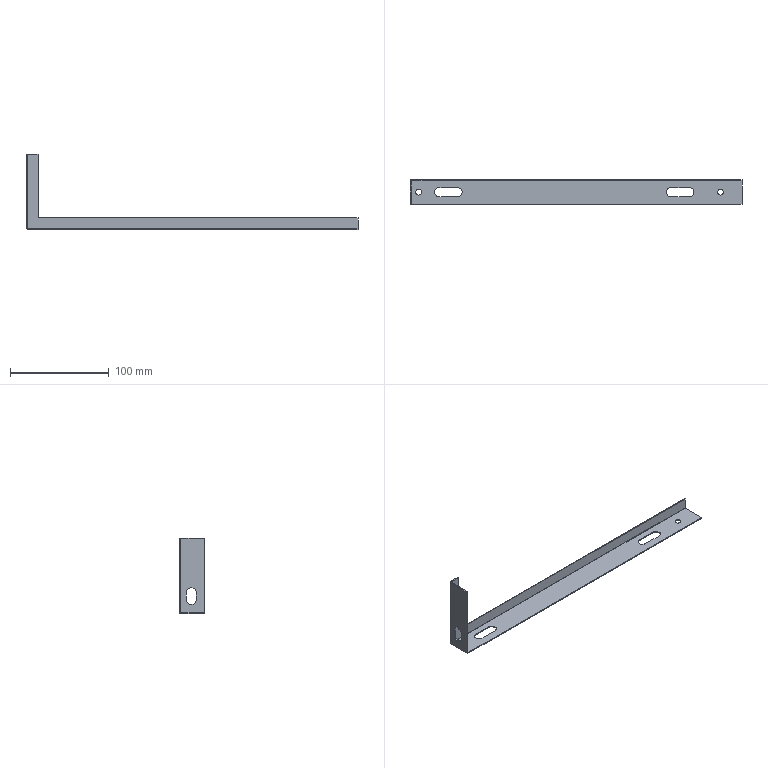Part | SolidWorks | features Cut 2, EdgeFlange 2, FlatPattern 1, ICE 1, LPattern 1, SMBaseFlange 1, SheetMetal 1 | 1 solid | 40 faces | box 336 x 25 x 76.7 mm | volume 13934 mm3 | plane 26 | cylinder 14 | commonest cylinder face diameters 6 x4 9 x4 0.4 x2 2.4 x2 10 x2
STEP:
#1=CARTESIAN_POINT('',(145.7,-15.5,-0.2));
#2=VERTEX_POINT('',#1);
#3=CARTESIAN_POINT('',(145.7,-9.5,-0.2));
#4=VERTEX_POINT('',#3);
#5=CARTESIAN_POINT('',(145.7,-12.5,-0.2));
#6=DIRECTION('',(0.,0.,-1.));
#7=DIRECTION('',(0.,1.,0.));
#8=AXIS2_PLACEMENT_3D('',#5,#6,#7);
#9=CIRCLE('',#8,3.);
#10=EDGE_CURVE('',#2,#4,#9,.T.);
#11=ORIENTED_EDGE('',*,*,#10,.F.);
#12=CARTESIAN_POINT('',(145.7,-15.5,-1.2));
#13=VERTEX_POINT('',#12);
#14=CARTESIAN_POINT('',(145.7,-15.5,8.8));
#15=DIRECTION('',(0.,0.,-1.));
#16=VECTOR('',#15,1000.);
#17=LINE('',#14,#16);
#18=EDGE_CURVE('',#2,#13,#17,.T.);
#19=ORIENTED_EDGE('',*,*,#18,.T.);
#20=CARTESIAN_POINT('',(145.7,-9.5,-1.2));
#21=VERTEX_POINT('',#20);
#22=CARTESIAN_POINT('',(145.7,-12.5,-1.2));
#23=DIRECTION('',(0.,0.,-1.));
#24=DIRECTION('',(0.,1.,0.));
#25=AXIS2_PLACEMENT_3D('',#22,#23,#24);
#26=CIRCLE('',#25,3.);
#27=EDGE_CURVE('',#13,#21,#26,.T.);
#28=ORIENTED_EDGE('',*,*,#27,.T.);
#29=CARTESIAN_POINT('',(145.7,-9.5,8.8));
#30=DIRECTION('',(0.,0.,-1.));
#31=VECTOR('',#30,1000.);
#32=LINE('',#29,#31);
#33=EDGE_CURVE('',#4,#21,#32,.T.);
#34=ORIENTED_EDGE('',*,*,#33,.F.);
#35=EDGE_LOOP('',(#11,#19,#28,#34));
#36=FACE_OUTER_BOUND('',#35,.T.);
#37=CARTESIAN_POINT('',(145.7,-12.5,8.8));
#38=DIRECTION('',(0.,0.,-1.));
#39=DIRECTION('',(0.,1.,0.));
#40=AXIS2_PLACEMENT_3D('',#37,#38,#39);
#41=CYLINDRICAL_SURFACE('',#40,3.);
#42=ADVANCED_FACE('',(#36),#41,.F.);
#43=CARTESIAN_POINT('',(-159.8,-15.5,-0.2));
#44=VERTEX_POINT('',#43);
#45=CARTESIAN_POINT('',(-159.8,-9.5,-0.2));
#46=VERTEX_POINT('',#45);
#47=CARTESIAN_POINT('',(-159.8,-12.5,-0.2));
#48=DIRECTION('',(0.,0.,-1.));
#49=DIRECTION('',(0.,1.,0.));
#50=AXIS2_PLACEMENT_3D('',#47,#48,#49);
#51=CIRCLE('',#50,3.);
#52=EDGE_CURVE('',#44,#46,#51,.T.);
#53=ORIENTED_EDGE('',*,*,#52,.F.);
#54=CARTESIAN_POINT('',(-159.8,-15.5,-1.2));
#55=VERTEX_POINT('',#54);
#56=CARTESIAN_POINT('',(-159.8,-15.5,8.8));
#57=DIRECTION('',(0.,0.,-1.));
#58=VECTOR('',#57,1000.);
#59=LINE('',#56,#58);
#60=EDGE_CURVE('',#44,#55,#59,.T.);
#61=ORIENTED_EDGE('',*,*,#60,.T.);
#62=CARTESIAN_POINT('',(-159.8,-9.5,-1.2));
#63=VERTEX_POINT('',#62);
#64=CARTESIAN_POINT('',(-159.8,-12.5,-1.2));
#65=DIRECTION('',(0.,0.,-1.));
#66=DIRECTION('',(0.,1.,0.));
#67=AXIS2_PLACEMENT_3D('',#64,#65,#66);
#68=CIRCLE('',#67,3.);
#69=EDGE_CURVE('',#55,#63,#68,.T.);
#70=ORIENTED_EDGE('',*,*,#69,.T.);
#71=CARTESIAN_POINT('',(-159.8,-9.5,8.8));
#72=DIRECTION('',(0.,0.,-1.));
#73=VECTOR('',#72,1000.);
#74=LINE('',#71,#73);
#75=EDGE_CURVE('',#46,#63,#74,.T.);
#76=ORIENTED_EDGE('',*,*,#75,.F.);
#77=EDGE_LOOP('',(#53,#61,#70,#76));
#78=FACE_OUTER_BOUND('',#77,.T.);
#79=CARTESIAN_POINT('',(-159.8,-12.5,8.8));
#80=DIRECTION('',(0.,0.,-1.));
#81=DIRECTION('',(0.,1.,0.));
#82=AXIS2_PLACEMENT_3D('',#79,#80,#81);
#83=CYLINDRICAL_SURFACE('',#82,3.);
#84=ADVANCED_FACE('',(#78),#83,.F.);
#85=CARTESIAN_POINT('',(167.4,-1.,11.));
#86=VERTEX_POINT('',#85);
#87=CARTESIAN_POINT('',(-156.4,-1.,11.));
#88=VERTEX_POINT('',#87);
#89=CARTESIAN_POINT('',(-167.4,-1.,11.));
#90=DIRECTION('',(-1.,0.,0.));
#91=VECTOR('',#90,1000.);
#92=LINE('',#89,#91);
#93=EDGE_CURVE('',#86,#88,#92,.T.);
#94=ORIENTED_EDGE('',*,*,#93,.T.);
#95=CARTESIAN_POINT('',(-156.4,-1.,75.5));
#96=VERTEX_POINT('',#95);
#97=CARTESIAN_POINT('',(-156.4,-1.,75.5));
#98=DIRECTION('',(0.,0.,1.));
#99=VECTOR('',#98,1000.);
#100=LINE('',#97,#99);
#101=EDGE_CURVE('',#88,#96,#100,.T.);
#102=ORIENTED_EDGE('',*,*,#101,.T.);
#103=CARTESIAN_POINT('',(-167.4,-1.,75.5));
#104=VERTEX_POINT('',#103);
#105=CARTESIAN_POINT('',(-167.4,-1.,75.5));
#106=DIRECTION('',(1.,0.,0.));
#107=VECTOR('',#106,1000.);
#108=LINE('',#105,#107);
#109=EDGE_CURVE('',#104,#96,#108,.T.);
#110=ORIENTED_EDGE('',*,*,#109,.F.);
#111=CARTESIAN_POINT('',(-167.4,-1.,0.));
#112=VERTEX_POINT('',#111);
#113=CARTESIAN_POINT('',(-167.4,-1.,75.5));
#114=DIRECTION('',(0.,0.,-1.));
#115=VECTOR('',#114,1000.);
#116=LINE('',#113,#115);
#117=EDGE_CURVE('',#104,#112,#116,.T.);
#118=ORIENTED_EDGE('',*,*,#117,.T.);
#119=CARTESIAN_POINT('',(167.4,-1.,0.));
#120=VERTEX_POINT('',#119);
#121=CARTESIAN_POINT('',(-167.4,-1.,0.));
#122=DIRECTION('',(1.,0.,0.));
#123=VECTOR('',#122,1000.);
#124=LINE('',#121,#123);
#125=EDGE_CURVE('',#112,#120,#124,.T.);
#126=ORIENTED_EDGE('',*,*,#125,.T.);
#127=CARTESIAN_POINT('',(167.4,-1.,75.5));
#128=DIRECTION('',(0.,0.,-1.));
#129=VECTOR('',#128,1000.);
#130=LINE('',#127,#129);
#131=EDGE_CURVE('',#86,#120,#130,.T.);
#132=ORIENTED_EDGE('',*,*,#131,.F.);
#133=EDGE_LOOP('',(#94,#102,#110,#118,#126,#132));
#134=FACE_OUTER_BOUND('',#133,.T.);
#135=CARTESIAN_POINT('',(-167.4,-1.,75.5));
#136=DIRECTION('',(0.,1.,0.));
#137=DIRECTION('',(-1.,0.,0.));
#138=AXIS2_PLACEMENT_3D('',#135,#136,#137);
#139=PLANE('',#138);
#140=ADVANCED_FACE('',(#134),#139,.F.);
#141=CARTESIAN_POINT('',(167.4,0.,11.));
#142=VERTEX_POINT('',#141);
#143=CARTESIAN_POINT('',(167.4,-10.,11.));
#144=DIRECTION('',(0.,1.,0.));
#145=VECTOR('',#144,1000.);
#146=LINE('',#143,#145);
#147=EDGE_CURVE('',#86,#142,#146,.T.);
#148=ORIENTED_EDGE('',*,*,#147,.F.);
#149=ORIENTED_EDGE('',*,*,#131,.T.);
#150=CARTESIAN_POINT('',(167.4,0.,0.));
#151=VERTEX_POINT('',#150);
#152=CARTESIAN_POINT('',(167.4,0.,0.));
#153=DIRECTION('',(0.,-1.,0.));
#154=VECTOR('',#153,1000.);
#155=LINE('',#152,#154);
#156=EDGE_CURVE('',#151,#120,#155,.T.);
#157=ORIENTED_EDGE('',*,*,#156,.F.);
#158=CARTESIAN_POINT('',(167.4,0.,75.5));
#159=DIRECTION('',(0.,0.,-1.));
#160=VECTOR('',#159,1000.);
#161=LINE('',#158,#160);
#162=EDGE_CURVE('',#142,#151,#161,.T.);
#163=ORIENTED_EDGE('',*,*,#162,.F.);
#164=EDGE_LOOP('',(#148,#149,#157,#163));
#165=FACE_OUTER_BOUND('',#164,.T.);
#166=CARTESIAN_POINT('',(167.4,0.,75.5));
#167=DIRECTION('',(1.,0.,0.));
#168=DIRECTION('',(0.,0.,-1.));
#169=AXIS2_PLACEMENT_3D('',#166,#167,#168);
#170=PLANE('',#169);
#171=ADVANCED_FACE('',(#165),#170,.T.);
#172=CARTESIAN_POINT('',(-156.4,0.,11.));
#173=VERTEX_POINT('',#172);
#174=CARTESIAN_POINT('',(-156.4,0.,75.5));
#175=VERTEX_POINT('',#174);
#176=CARTESIAN_POINT('',(-156.4,0.,75.5));
#177=DIRECTION('',(0.,0.,1.));
#178=VECTOR('',#177,1000.);
#179=LINE('',#176,#178);
#180=EDGE_CURVE('',#173,#175,#179,.T.);
#181=ORIENTED_EDGE('',*,*,#180,.F.);
#182=CARTESIAN_POINT('',(167.4,0.,11.));
#183=DIRECTION('',(-1.,0.,0.));
#184=VECTOR('',#183,1000.);
#185=LINE('',#182,#184);
#186=EDGE_CURVE('',#142,#173,#185,.T.);
#187=ORIENTED_EDGE('',*,*,#186,.F.);
#188=ORIENTED_EDGE('',*,*,#162,.T.);
#189=CARTESIAN_POINT('',(-167.4,0.,0.));
#190=VERTEX_POINT('',#189);
#191=CARTESIAN_POINT('',(-167.4,0.,0.));
#192=DIRECTION('',(1.,0.,0.));
#193=VECTOR('',#192,1000.);
#194=LINE('',#191,#193);
#195=EDGE_CURVE('',#190,#151,#194,.T.);
#196=ORIENTED_EDGE('',*,*,#195,.F.);
#197=CARTESIAN_POINT('',(-167.4,0.,75.5));
#198=VERTEX_POINT('',#197);
#199=CARTESIAN_POINT('',(-167.4,0.,75.5));
#200=DIRECTION('',(0.,0.,-1.));
#201=VECTOR('',#200,1000.);
#202=LINE('',#199,#201);
#203=EDGE_CURVE('',#198,#190,#202,.T.);
#204=ORIENTED_EDGE('',*,*,#203,.F.);
#205=CARTESIAN_POINT('',(-167.4,0.,75.5));
#206=DIRECTION('',(1.,0.,0.));
#207=VECTOR('',#206,1000.);
#208=LINE('',#205,#207);
#209=EDGE_CURVE('',#198,#175,#208,.T.);
#210=ORIENTED_EDGE('',*,*,#209,.T.);
#211=EDGE_LOOP('',(#181,#187,#188,#196,#204,#210));
#212=FACE_OUTER_BOUND('',#211,.T.);
#213=CARTESIAN_POINT('',(-167.4,0.,75.5));
#214=DIRECTION('',(0.,1.,0.));
#215=DIRECTION('',(-1.,0.,0.));
#216=AXIS2_PLACEMENT_3D('',#213,#214,#215);
#217=PLANE('',#216);
#218=ADVANCED_FACE('',(#212),#217,.T.);
#219=ORIENTED_EDGE('',*,*,#109,.T.);
#220=CARTESIAN_POINT('',(-156.4,0.,75.5));
#221=DIRECTION('',(0.,1.,0.));
#222=VECTOR('',#221,1000.);
#223=LINE('',#220,#222);
#224=EDGE_CURVE('',#96,#175,#223,.T.);
#225=ORIENTED_EDGE('',*,*,#224,.T.);
#226=ORIENTED_EDGE('',*,*,#209,.F.);
#227=CARTESIAN_POINT('',(-167.4,-1.,75.5));
#228=DIRECTION('',(0.,1.,0.));
#229=VECTOR('',#228,1000.);
#230=LINE('',#227,#229);
#231=EDGE_CURVE('',#104,#198,#230,.T.);
#232=ORIENTED_EDGE('',*,*,#231,.F.);
#233=EDGE_LOOP('',(#219,#225,#226,#232));
#234=FACE_OUTER_BOUND('',#233,.T.);
#235=CARTESIAN_POINT('',(0.,0.,75.5));
#236=DIRECTION('',(0.,0.,-1.));
#237=DIRECTION('',(-1.,0.,0.));
#238=AXIS2_PLACEMENT_3D('',#235,#236,#237);
#239=PLANE('',#238);
#240=ADVANCED_FACE('',(#234),#239,.F.);
#241=ORIENTED_EDGE('',*,*,#147,.T.);
#242=ORIENTED_EDGE('',*,*,#186,.T.);
#243=CARTESIAN_POINT('',(-156.4,-10.,11.));
#244=DIRECTION('',(0.,1.,0.));
#245=VECTOR('',#244,1000.);
#246=LINE('',#243,#245);
#247=EDGE_CURVE('',#88,#173,#246,.T.);
#248=ORIENTED_EDGE('',*,*,#247,.F.);
#249=ORIENTED_EDGE('',*,*,#93,.F.);
#250=EDGE_LOOP('',(#241,#242,#248,#249));
#251=FACE_OUTER_BOUND('',#250,.T.);
#252=CARTESIAN_POINT('',(167.4,-10.,11.));
#253=DIRECTION('',(0.,0.,-1.));
#254=DIRECTION('',(-1.,0.,0.));
#255=AXIS2_PLACEMENT_3D('',#252,#253,#254);
#256=PLANE('',#255);
#257=ADVANCED_FACE('',(#251),#256,.F.);
#258=ORIENTED_EDGE('',*,*,#247,.T.);
#259=ORIENTED_EDGE('',*,*,#180,.T.);
#260=ORIENTED_EDGE('',*,*,#224,.F.);
#261=ORIENTED_EDGE('',*,*,#101,.F.);
#262=EDGE_LOOP('',(#258,#259,#260,#261));
#263=FACE_OUTER_BOUND('',#262,.T.);
#264=CARTESIAN_POINT('',(-156.4,-10.,75.5));
#265=DIRECTION('',(-1.,0.,0.));
#266=DIRECTION('',(0.,0.,1.));
#267=AXIS2_PLACEMENT_3D('',#264,#265,#266);
#268=PLANE('',#267);
#269=ADVANCED_FACE('',(#263),#268,.F.);
#270=CARTESIAN_POINT('',(-167.4,-1.2,-0.2));
#271=VERTEX_POINT('',#270);
#272=CARTESIAN_POINT('',(-167.4,-1.2,-1.2));
#273=VERTEX_POINT('',#272);
#274=CARTESIAN_POINT('',(-167.4,-1.2,-1.2));
#275=DIRECTION('',(0.,0.,-1.));
#276=VECTOR('',#275,1000.);
#277=LINE('',#274,#276);
#278=EDGE_CURVE('',#271,#273,#277,.T.);
#279=ORIENTED_EDGE('',*,*,#278,.F.);
#280=CARTESIAN_POINT('',(-167.4,-1.2,0.));
#281=DIRECTION('',(-1.,0.,0.));
#282=DIRECTION('',(0.,1.,0.));
#283=AXIS2_PLACEMENT_3D('',#280,#281,#282);
#284=CIRCLE('',#283,0.2);
#285=EDGE_CURVE('',#112,#271,#284,.T.);
#286=ORIENTED_EDGE('',*,*,#285,.F.);
#287=CARTESIAN_POINT('',(-167.4,-1.,0.));
#288=DIRECTION('',(0.,1.,0.));
#289=VECTOR('',#288,1000.);
#290=LINE('',#287,#289);
#291=EDGE_CURVE('',#112,#190,#290,.T.);
#292=ORIENTED_EDGE('',*,*,#291,.T.);
#293=CARTESIAN_POINT('',(-167.4,-1.2,0.));
#294=DIRECTION('',(-1.,0.,0.));
#295=DIRECTION('',(0.,1.,0.));
#296=AXIS2_PLACEMENT_3D('',#293,#294,#295);
#297=CIRCLE('',#296,1.2);
#298=EDGE_CURVE('',#190,#273,#297,.T.);
#299=ORIENTED_EDGE('',*,*,#298,.T.);
#300=EDGE_LOOP('',(#279,#286,#292,#299));
#301=FACE_OUTER_BOUND('',#300,.T.);
#302=CARTESIAN_POINT('',(-167.4,-1.2,0.));
#303=DIRECTION('',(-1.,0.,0.));
#304=DIRECTION('',(0.,-1.,0.));
#305=AXIS2_PLACEMENT_3D('',#302,#303,#304);
#306=PLANE('',#305);
#307=ADVANCED_FACE('',(#301),#306,.T.);
#308=CARTESIAN_POINT('',(167.4,-1.2,-0.2));
#309=VERTEX_POINT('',#308);
#310=CARTESIAN_POINT('',(167.4,-1.2,0.));
#311=DIRECTION('',(1.,0.,0.));
#312=DIRECTION('',(0.,1.,0.));
#313=AXIS2_PLACEMENT_3D('',#310,#311,#312);
#314=CIRCLE('',#313,0.2);
#315=EDGE_CURVE('',#309,#120,#314,.T.);
#316=ORIENTED_EDGE('',*,*,#315,.F.);
#317=CARTESIAN_POINT('',(167.4,-1.2,-1.2));
#318=VERTEX_POINT('',#317);
#319=CARTESIAN_POINT('',(167.4,-1.2,-0.2));
#320=DIRECTION('',(0.,0.,-1.));
#321=VECTOR('',#320,1000.);
#322=LINE('',#319,#321);
#323=EDGE_CURVE('',#309,#318,#322,.T.);
#324=ORIENTED_EDGE('',*,*,#323,.T.);
#325=CARTESIAN_POINT('',(167.4,-1.2,0.));
#326=DIRECTION('',(1.,0.,0.));
#327=DIRECTION('',(0.,1.,0.));
#328=AXIS2_PLACEMENT_3D('',#325,#326,#327);
#329=CIRCLE('',#328,1.2);
#330=EDGE_CURVE('',#318,#151,#329,.T.);
#331=ORIENTED_EDGE('',*,*,#330,.T.);
#332=ORIENTED_EDGE('',*,*,#156,.T.);
#333=EDGE_LOOP('',(#316,#324,#331,#332));
#334=FACE_OUTER_BOUND('',#333,.T.);
#335=CARTESIAN_POINT('',(167.4,-1.2,0.));
#336=DIRECTION('',(-1.,0.,0.));
#337=DIRECTION('',(0.,-1.,0.));
#338=AXIS2_PLACEMENT_3D('',#335,#336,#337);
#339=PLANE('',#338);
#340=ADVANCED_FACE('',(#334),#339,.F.);
#341=ORIENTED_EDGE('',*,*,#195,.T.);
#342=ORIENTED_EDGE('',*,*,#330,.F.);
#343=CARTESIAN_POINT('',(0.,-1.2,-1.2));
#344=DIRECTION('',(1.,0.,0.));
#345=VECTOR('',#344,1000.);
#346=LINE('',#343,#345);
#347=EDGE_CURVE('',#273,#318,#346,.T.);
#348=ORIENTED_EDGE('',*,*,#347,.F.);
#349=ORIENTED_EDGE('',*,*,#298,.F.);
#350=EDGE_LOOP('',(#341,#342,#348,#349));
#351=FACE_OUTER_BOUND('',#350,.T.);
#352=CARTESIAN_POINT('',(167.4,-1.2,0.));
#353=DIRECTION('',(1.,0.,0.));
#354=DIRECTION('',(0.,0.,-1.));
#355=AXIS2_PLACEMENT_3D('',#352,#353,#354);
#356=CYLINDRICAL_SURFACE('',#355,1.2);
#357=ADVANCED_FACE('',(#351),#356,.T.);
#358=ORIENTED_EDGE('',*,*,#125,.F.);
#359=ORIENTED_EDGE('',*,*,#285,.T.);
#360=CARTESIAN_POINT('',(-167.4,-1.2,-0.2));
#361=DIRECTION('',(1.,0.,0.));
#362=VECTOR('',#361,1000.);
#363=LINE('',#360,#362);
#364=EDGE_CURVE('',#271,#309,#363,.T.);
#365=ORIENTED_EDGE('',*,*,#364,.T.);
#366=ORIENTED_EDGE('',*,*,#315,.T.);
#367=EDGE_LOOP('',(#358,#359,#365,#366));
#368=FACE_OUTER_BOUND('',#367,.T.);
#369=CARTESIAN_POINT('',(167.4,-1.2,0.));
#370=DIRECTION('',(1.,0.,0.));
#371=DIRECTION('',(0.,0.,-1.));
#372=AXIS2_PLACEMENT_3D('',#369,#370,#371);
#373=CYLINDRICAL_SURFACE('',#372,0.2);
#374=ADVANCED_FACE('',(#368),#373,.F.);
#375=CARTESIAN_POINT('',(167.4,-25.,-1.2));
#376=VERTEX_POINT('',#375);
#377=CARTESIAN_POINT('',(167.4,-1.,-1.2));
#378=DIRECTION('',(0.,1.,0.));
#379=VECTOR('',#378,1000.);
#380=LINE('',#377,#379);
#381=EDGE_CURVE('',#376,#318,#380,.T.);
#382=ORIENTED_EDGE('',*,*,#381,.T.);
#383=ORIENTED_EDGE('',*,*,#323,.F.);
#384=CARTESIAN_POINT('',(167.4,-25.,-0.2));
#385=VERTEX_POINT('',#384);
#386=CARTESIAN_POINT('',(167.4,0.,-0.2));
#387=DIRECTION('',(0.,1.,0.));
#388=VECTOR('',#387,1000.);
#389=LINE('',#386,#388);
#390=EDGE_CURVE('',#385,#309,#389,.T.);
#391=ORIENTED_EDGE('',*,*,#390,.F.);
#392=CARTESIAN_POINT('',(167.4,-25.,-1.2));
#393=DIRECTION('',(0.,0.,1.));
#394=VECTOR('',#393,1000.);
#395=LINE('',#392,#394);
#396=EDGE_CURVE('',#376,#385,#395,.T.);
#397=ORIENTED_EDGE('',*,*,#396,.F.);
#398=EDGE_LOOP('',(#382,#383,#391,#397));
#399=FACE_OUTER_BOUND('',#398,.T.);
#400=CARTESIAN_POINT('',(167.4,-1.,-1.2));
#401=DIRECTION('',(1.,0.,0.));
#402=DIRECTION('',(0.,0.,-1.));
#403=AXIS2_PLACEMENT_3D('',#400,#401,#402);
#404=PLANE('',#403);
#405=ADVANCED_FACE('',(#399),#404,.T.);
#406=CARTESIAN_POINT('',(-167.4,-25.,-0.2));
#407=VERTEX_POINT('',#406);
#408=CARTESIAN_POINT('',(-167.4,0.,-0.2));
#409=DIRECTION('',(0.,-1.,0.));
#410=VECTOR('',#409,1000.);
#411=LINE('',#408,#410);
#412=EDGE_CURVE('',#271,#407,#411,.T.);
#413=ORIENTED_EDGE('',*,*,#412,.F.);
#414=ORIENTED_EDGE('',*,*,#278,.T.);
#415=CARTESIAN_POINT('',(-167.4,-25.,-1.2));
#416=VERTEX_POINT('',#415);
#417=CARTESIAN_POINT('',(-167.4,-25.,-1.2));
#418=DIRECTION('',(0.,-1.,0.));
#419=VECTOR('',#418,1000.);
#420=LINE('',#417,#419);
#421=EDGE_CURVE('',#273,#416,#420,.T.);
#422=ORIENTED_EDGE('',*,*,#421,.T.);
#423=CARTESIAN_POINT('',(-167.4,-25.,-1.2));
#424=DIRECTION('',(0.,0.,1.));
#425=VECTOR('',#424,1000.);
#426=LINE('',#423,#425);
#427=EDGE_CURVE('',#416,#407,#426,.T.);
#428=ORIENTED_EDGE('',*,*,#427,.T.);
#429=EDGE_LOOP('',(#413,#414,#422,#428));
#430=FACE_OUTER_BOUND('',#429,.T.);
#431=CARTESIAN_POINT('',(-167.4,-25.,-1.2));
#432=DIRECTION('',(-1.,0.,0.));
#433=DIRECTION('',(0.,0.,1.));
#434=AXIS2_PLACEMENT_3D('',#431,#432,#433);
#435=PLANE('',#434);
#436=ADVANCED_FACE('',(#430),#435,.T.);
#437=CARTESIAN_POINT('',(145.7,-12.5,-1.2));
#438=DIRECTION('',(0.,0.,-1.));
#439=DIRECTION('',(0.,1.,0.));
#440=AXIS2_PLACEMENT_3D('',#437,#438,#439);
#441=CIRCLE('',#440,3.);
#442=EDGE_CURVE('',#21,#13,#441,.T.);
#443=ORIENTED_EDGE('',*,*,#442,.F.);
#444=ORIENTED_EDGE('',*,*,#27,.F.);
#445=EDGE_LOOP('',(#443,#444));
#446=FACE_BOUND('',#445,.T.);
#447=CARTESIAN_POINT('',(-159.8,-12.5,-1.2));
#448=DIRECTION('',(0.,0.,-1.));
#449=DIRECTION('',(0.,1.,0.));
#450=AXIS2_PLACEMENT_3D('',#447,#448,#449);
#451=CIRCLE('',#450,3.);
#452=EDGE_CURVE('',#63,#55,#451,.T.);
#453=ORIENTED_EDGE('',*,*,#452,.F.);
#454=ORIENTED_EDGE('',*,*,#69,.F.);
#455=EDGE_LOOP('',(#453,#454));
#456=FACE_BOUND('',#455,.T.);
#457=CARTESIAN_POINT('',(95.2,-17.,-1.2));
#458=VERTEX_POINT('',#457);
#459=CARTESIAN_POINT('',(95.2,-8.,-1.2));
#460=VERTEX_POINT('',#459);
#461=CARTESIAN_POINT('',(95.2,-12.5,-1.2));
#462=DIRECTION('',(0.,0.,-1.));
#463=DIRECTION('',(0.,1.,0.));
#464=AXIS2_PLACEMENT_3D('',#461,#462,#463);
#465=CIRCLE('',#464,4.5);
#466=EDGE_CURVE('',#458,#460,#465,.T.);
#467=ORIENTED_EDGE('',*,*,#466,.F.);
#468=CARTESIAN_POINT('',(114.2,-17.,-1.2));
#469=VERTEX_POINT('',#468);
#470=CARTESIAN_POINT('',(95.2,-17.,-1.2));
#471=DIRECTION('',(-1.,0.,0.));
#472=VECTOR('',#471,1000.);
#473=LINE('',#470,#472);
#474=EDGE_CURVE('',#469,#458,#473,.T.);
#475=ORIENTED_EDGE('',*,*,#474,.F.);
#476=CARTESIAN_POINT('',(114.2,-8.,-1.2));
#477=VERTEX_POINT('',#476);
#478=CARTESIAN_POINT('',(114.2,-12.5,-1.2));
#479=DIRECTION('',(0.,0.,-1.));
#480=DIRECTION('',(0.,1.,0.));
#481=AXIS2_PLACEMENT_3D('',#478,#479,#480);
#482=CIRCLE('',#481,4.5);
#483=EDGE_CURVE('',#477,#469,#482,.T.);
#484=ORIENTED_EDGE('',*,*,#483,.F.);
#485=CARTESIAN_POINT('',(95.2,-8.,-1.2));
#486=DIRECTION('',(1.,0.,0.));
#487=VECTOR('',#486,1000.);
#488=LINE('',#485,#487);
#489=EDGE_CURVE('',#460,#477,#488,.T.);
#490=ORIENTED_EDGE('',*,*,#489,.F.);
#491=EDGE_LOOP('',(#467,#475,#484,#490));
#492=FACE_BOUND('',#491,.T.);
#493=CARTESIAN_POINT('',(-139.3,-17.,-1.2));
#494=VERTEX_POINT('',#493);
#495=CARTESIAN_POINT('',(-139.3,-8.,-1.2));
#496=VERTEX_POINT('',#495);
#497=CARTESIAN_POINT('',(-139.3,-12.5,-1.2));
#498=DIRECTION('',(0.,0.,-1.));
#499=DIRECTION('',(0.,1.,0.));
#500=AXIS2_PLACEMENT_3D('',#497,#498,#499);
#501=CIRCLE('',#500,4.5);
#502=EDGE_CURVE('',#494,#496,#501,.T.);
#503=ORIENTED_EDGE('',*,*,#502,.F.);
#504=CARTESIAN_POINT('',(-120.3,-17.,-1.2));
#505=VERTEX_POINT('',#504);
#506=CARTESIAN_POINT('',(-139.3,-17.,-1.2));
#507=DIRECTION('',(-1.,0.,0.));
#508=VECTOR('',#507,1000.);
#509=LINE('',#506,#508);
#510=EDGE_CURVE('',#505,#494,#509,.T.);
#511=ORIENTED_EDGE('',*,*,#510,.F.);
#512=CARTESIAN_POINT('',(-120.3,-8.,-1.2));
#513=VERTEX_POINT('',#512);
#514=CARTESIAN_POINT('',(-120.3,-12.5,-1.2));
#515=DIRECTION('',(0.,0.,-1.));
#516=DIRECTION('',(0.,1.,0.));
#517=AXIS2_PLACEMENT_3D('',#514,#515,#516);
#518=CIRCLE('',#517,4.5);
#519=EDGE_CURVE('',#513,#505,#518,.T.);
#520=ORIENTED_EDGE('',*,*,#519,.F.);
#521=CARTESIAN_POINT('',(-139.3,-8.,-1.2));
#522=DIRECTION('',(1.,0.,0.));
#523=VECTOR('',#522,1000.);
#524=LINE('',#521,#523);
#525=EDGE_CURVE('',#496,#513,#524,.T.);
#526=ORIENTED_EDGE('',*,*,#525,.F.);
#527=EDGE_LOOP('',(#503,#511,#520,#526));
#528=FACE_BOUND('',#527,.T.);
#529=ORIENTED_EDGE('',*,*,#421,.F.);
#530=ORIENTED_EDGE('',*,*,#347,.T.);
#531=ORIENTED_EDGE('',*,*,#381,.F.);
#532=CARTESIAN_POINT('',(167.4,-25.,-1.2));
#533=DIRECTION('',(1.,0.,0.));
#534=VECTOR('',#533,1000.);
#535=LINE('',#532,#534);
#536=EDGE_CURVE('',#416,#376,#535,.T.);
#537=ORIENTED_EDGE('',*,*,#536,.F.);
#538=EDGE_LOOP('',(#529,#530,#531,#537));
#539=FACE_OUTER_BOUND('',#538,.T.);
#540=CARTESIAN_POINT('',(0.,0.,-1.2));
#541=DIRECTION('',(0.,0.,-1.));
#542=DIRECTION('',(0.,1.,0.));
#543=AXIS2_PLACEMENT_3D('',#540,#541,#542);
#544=PLANE('',#543);
#545=ADVANCED_FACE('',(#446,#456,#492,#528,#539),#544,.T.);
#546=CARTESIAN_POINT('',(145.7,-12.5,-0.2));
#547=DIRECTION('',(0.,0.,-1.));
#548=DIRECTION('',(0.,1.,0.));
#549=AXIS2_PLACEMENT_3D('',#546,#547,#548);
#550=CIRCLE('',#549,3.);
#551=EDGE_CURVE('',#4,#2,#550,.T.);
#552=ORIENTED_EDGE('',*,*,#551,.T.);
#553=ORIENTED_EDGE('',*,*,#10,.T.);
#554=EDGE_LOOP('',(#552,#553));
#555=FACE_BOUND('',#554,.T.);
#556=CARTESIAN_POINT('',(-159.8,-12.5,-0.2));
#557=DIRECTION('',(0.,0.,-1.));
#558=DIRECTION('',(0.,1.,0.));
#559=AXIS2_PLACEMENT_3D('',#556,#557,#558);
#560=CIRCLE('',#559,3.);
#561=EDGE_CURVE('',#46,#44,#560,.T.);
#562=ORIENTED_EDGE('',*,*,#561,.T.);
#563=ORIENTED_EDGE('',*,*,#52,.T.);
#564=EDGE_LOOP('',(#562,#563));
#565=FACE_BOUND('',#564,.T.);
#566=CARTESIAN_POINT('',(114.2,-17.,-0.2));
#567=VERTEX_POINT('',#566);
#568=CARTESIAN_POINT('',(95.2,-17.,-0.2));
#569=VERTEX_POINT('',#568);
#570=CARTESIAN_POINT('',(0.,-17.,-0.2));
#571=DIRECTION('',(-1.,0.,0.));
#572=VECTOR('',#571,1000.);
#573=LINE('',#570,#572);
#574=EDGE_CURVE('',#567,#569,#573,.T.);
#575=ORIENTED_EDGE('',*,*,#574,.T.);
#576=CARTESIAN_POINT('',(95.2,-8.,-0.2));
#577=VERTEX_POINT('',#576);
#578=CARTESIAN_POINT('',(95.2,-12.5,-0.2));
#579=DIRECTION('',(0.,0.,-1.));
#580=DIRECTION('',(0.,1.,0.));
#581=AXIS2_PLACEMENT_3D('',#578,#579,#580);
#582=CIRCLE('',#581,4.5);
#583=EDGE_CURVE('',#569,#577,#582,.T.);
#584=ORIENTED_EDGE('',*,*,#583,.T.);
#585=CARTESIAN_POINT('',(114.2,-8.,-0.2));
#586=VERTEX_POINT('',#585);
#587=CARTESIAN_POINT('',(0.,-8.,-0.2));
#588=DIRECTION('',(1.,0.,0.));
#589=VECTOR('',#588,1000.);
#590=LINE('',#587,#589);
#591=EDGE_CURVE('',#577,#586,#590,.T.);
#592=ORIENTED_EDGE('',*,*,#591,.T.);
#593=CARTESIAN_POINT('',(114.2,-12.5,-0.2));
#594=DIRECTION('',(0.,0.,-1.));
#595=DIRECTION('',(0.,1.,0.));
#596=AXIS2_PLACEMENT_3D('',#593,#594,#595);
#597=CIRCLE('',#596,4.5);
#598=EDGE_CURVE('',#586,#567,#597,.T.);
#599=ORIENTED_EDGE('',*,*,#598,.T.);
#600=EDGE_LOOP('',(#575,#584,#592,#599));
#601=FACE_BOUND('',#600,.T.);
#602=CARTESIAN_POINT('',(-120.3,-17.,-0.2));
#603=VERTEX_POINT('',#602);
#604=CARTESIAN_POINT('',(-139.3,-17.,-0.2));
#605=VERTEX_POINT('',#604);
#606=CARTESIAN_POINT('',(0.,-17.,-0.2));
#607=DIRECTION('',(-1.,0.,0.));
#608=VECTOR('',#607,1000.);
#609=LINE('',#606,#608);
#610=EDGE_CURVE('',#603,#605,#609,.T.);
#611=ORIENTED_EDGE('',*,*,#610,.T.);
#612=CARTESIAN_POINT('',(-139.3,-8.,-0.2));
#613=VERTEX_POINT('',#612);
#614=CARTESIAN_POINT('',(-139.3,-12.5,-0.2));
#615=DIRECTION('',(0.,0.,-1.));
#616=DIRECTION('',(0.,1.,0.));
#617=AXIS2_PLACEMENT_3D('',#614,#615,#616);
#618=CIRCLE('',#617,4.5);
#619=EDGE_CURVE('',#605,#613,#618,.T.);
#620=ORIENTED_EDGE('',*,*,#619,.T.);
#621=CARTESIAN_POINT('',(-120.3,-8.,-0.2));
#622=VERTEX_POINT('',#621);
#623=CARTESIAN_POINT('',(0.,-8.,-0.2));
#624=DIRECTION('',(1.,0.,0.));
#625=VECTOR('',#624,1000.);
#626=LINE('',#623,#625);
#627=EDGE_CURVE('',#613,#622,#626,.T.);
#628=ORIENTED_EDGE('',*,*,#627,.T.);
#629=CARTESIAN_POINT('',(-120.3,-12.5,-0.2));
#630=DIRECTION('',(0.,0.,-1.));
#631=DIRECTION('',(0.,1.,0.));
#632=AXIS2_PLACEMENT_3D('',#629,#630,#631);
#633=CIRCLE('',#632,4.5);
#634=EDGE_CURVE('',#622,#603,#633,.T.);
#635=ORIENTED_EDGE('',*,*,#634,.T.);
#636=EDGE_LOOP('',(#611,#620,#628,#635));
#637=FACE_BOUND('',#636,.T.);
#638=ORIENTED_EDGE('',*,*,#364,.F.);
#639=ORIENTED_EDGE('',*,*,#412,.T.);
#640=CARTESIAN_POINT('',(0.,-25.,-0.2));
#641=DIRECTION('',(1.,0.,0.));
#642=VECTOR('',#641,1000.);
#643=LINE('',#640,#642);
#644=EDGE_CURVE('',#407,#385,#643,.T.);
#645=ORIENTED_EDGE('',*,*,#644,.T.);
#646=ORIENTED_EDGE('',*,*,#390,.T.);
#647=EDGE_LOOP('',(#638,#639,#645,#646));
#648=FACE_OUTER_BOUND('',#647,.T.);
#649=CARTESIAN_POINT('',(0.,0.,-0.2));
#650=DIRECTION('',(0.,0.,-1.));
#651=DIRECTION('',(0.,1.,0.));
#652=AXIS2_PLACEMENT_3D('',#649,#650,#651);
#653=PLANE('',#652);
#654=ADVANCED_FACE('',(#555,#565,#601,#637,#648),#653,.F.);
#655=ORIENTED_EDGE('',*,*,#644,.F.);
#656=ORIENTED_EDGE('',*,*,#427,.F.);
#657=ORIENTED_EDGE('',*,*,#536,.T.);
#658=ORIENTED_EDGE('',*,*,#396,.T.);
#659=EDGE_LOOP('',(#655,#656,#657,#658));
#660=FACE_OUTER_BOUND('',#659,.T.);
#661=CARTESIAN_POINT('',(167.4,-25.,-1.2));
#662=DIRECTION('',(0.,-1.,0.));
#663=DIRECTION('',(0.,0.,-1.));
#664=AXIS2_PLACEMENT_3D('',#661,#662,#663);
#665=PLANE('',#664);
#666=ADVANCED_FACE('',(#660),#665,.T.);
#667=CARTESIAN_POINT('',(-167.6,-1.2,75.5));
#668=VERTEX_POINT('',#667);
#669=CARTESIAN_POINT('',(-168.6,-1.2,75.5));
#670=VERTEX_POINT('',#669);
#671=CARTESIAN_POINT('',(-168.6,-1.2,75.5));
#672=DIRECTION('',(-1.,0.,0.));
#673=VECTOR('',#672,1000.);
#674=LINE('',#671,#673);
#675=EDGE_CURVE('',#668,#670,#674,.T.);
#676=ORIENTED_EDGE('',*,*,#675,.F.);
#677=CARTESIAN_POINT('',(-167.4,-1.2,75.5));
#678=DIRECTION('',(0.,0.,1.));
#679=DIRECTION('',(-1.,0.,0.));
#680=AXIS2_PLACEMENT_3D('',#677,#678,#679);
#681=CIRCLE('',#680,0.2);
#682=EDGE_CURVE('',#104,#668,#681,.T.);
#683=ORIENTED_EDGE('',*,*,#682,.F.);
#684=ORIENTED_EDGE('',*,*,#231,.T.);
#685=CARTESIAN_POINT('',(-167.4,-1.2,75.5));
#686=DIRECTION('',(0.,0.,1.));
#687=DIRECTION('',(-1.,0.,0.));
#688=AXIS2_PLACEMENT_3D('',#685,#686,#687);
#689=CIRCLE('',#688,1.2);
#690=EDGE_CURVE('',#198,#670,#689,.T.);
#691=ORIENTED_EDGE('',*,*,#690,.T.);
#692=EDGE_LOOP('',(#676,#683,#684,#691));
#693=FACE_OUTER_BOUND('',#692,.T.);
#694=CARTESIAN_POINT('',(-167.4,-1.2,75.5));
#695=DIRECTION('',(0.,0.,1.));
#696=DIRECTION('',(1.,0.,0.));
#697=AXIS2_PLACEMENT_3D('',#694,#695,#696);
#698=PLANE('',#697);
#699=ADVANCED_FACE('',(#693),#698,.T.);
#700=CARTESIAN_POINT('',(-167.6,-1.2,0.));
#701=VERTEX_POINT('',#700);
#702=CARTESIAN_POINT('',(-167.4,-1.2,0.));
#703=DIRECTION('',(0.,0.,-1.));
#704=DIRECTION('',(-1.,0.,0.));
#705=AXIS2_PLACEMENT_3D('',#702,#703,#704);
#706=CIRCLE('',#705,0.2);
#707=EDGE_CURVE('',#701,#112,#706,.T.);
#708=ORIENTED_EDGE('',*,*,#707,.F.);
#709=CARTESIAN_POINT('',(-168.6,-1.2,0.));
#710=VERTEX_POINT('',#709);
#711=CARTESIAN_POINT('',(-167.6,-1.2,0.));
#712=DIRECTION('',(-1.,0.,0.));
#713=VECTOR('',#712,1000.);
#714=LINE('',#711,#713);
#715=EDGE_CURVE('',#701,#710,#714,.T.);
#716=ORIENTED_EDGE('',*,*,#715,.T.);
#717=CARTESIAN_POINT('',(-167.4,-1.2,0.));
#718=DIRECTION('',(0.,0.,-1.));
#719=DIRECTION('',(-1.,0.,0.));
#720=AXIS2_PLACEMENT_3D('',#717,#718,#719);
#721=CIRCLE('',#720,1.2);
#722=EDGE_CURVE('',#710,#190,#721,.T.);
#723=ORIENTED_EDGE('',*,*,#722,.T.);
#724=ORIENTED_EDGE('',*,*,#291,.F.);
#725=EDGE_LOOP('',(#708,#716,#723,#724));
#726=FACE_OUTER_BOUND('',#725,.T.);
#727=CARTESIAN_POINT('',(-167.4,-1.2,0.));
#728=DIRECTION('',(0.,0.,1.));
#729=DIRECTION('',(1.,0.,0.));
#730=AXIS2_PLACEMENT_3D('',#727,#728,#729);
#731=PLANE('',#730);
#732=ADVANCED_FACE('',(#726),#731,.F.);
#733=ORIENTED_EDGE('',*,*,#203,.T.);
#734=ORIENTED_EDGE('',*,*,#722,.F.);
#735=CARTESIAN_POINT('',(-168.6,-1.2,0.));
#736=DIRECTION('',(0.,0.,-1.));
#737=VECTOR('',#736,1000.);
#738=LINE('',#735,#737);
#739=EDGE_CURVE('',#670,#710,#738,.T.);
#740=ORIENTED_EDGE('',*,*,#739,.F.);
#741=ORIENTED_EDGE('',*,*,#690,.F.);
#742=EDGE_LOOP('',(#733,#734,#740,#741));
#743=FACE_OUTER_BOUND('',#742,.T.);
#744=CARTESIAN_POINT('',(-167.4,-1.2,0.));
#745=DIRECTION('',(0.,0.,-1.));
#746=DIRECTION('',(-1.,0.,0.));
#747=AXIS2_PLACEMENT_3D('',#744,#745,#746);
#748=CYLINDRICAL_SURFACE('',#747,1.2);
#749=ADVANCED_FACE('',(#743),#748,.T.);
#750=ORIENTED_EDGE('',*,*,#117,.F.);
#751=ORIENTED_EDGE('',*,*,#682,.T.);
#752=CARTESIAN_POINT('',(-167.6,-1.2,75.5));
#753=DIRECTION('',(0.,0.,-1.));
#754=VECTOR('',#753,1000.);
#755=LINE('',#752,#754);
#756=EDGE_CURVE('',#668,#701,#755,.T.);
#757=ORIENTED_EDGE('',*,*,#756,.T.);
#758=ORIENTED_EDGE('',*,*,#707,.T.);
#759=EDGE_LOOP('',(#750,#751,#757,#758));
#760=FACE_OUTER_BOUND('',#759,.T.);
#761=CARTESIAN_POINT('',(-167.4,-1.2,0.));
#762=DIRECTION('',(0.,0.,-1.));
#763=DIRECTION('',(-1.,0.,0.));
#764=AXIS2_PLACEMENT_3D('',#761,#762,#763);
#765=CYLINDRICAL_SURFACE('',#764,0.2);
#766=ADVANCED_FACE('',(#760),#765,.F.);
#767=CARTESIAN_POINT('',(-168.6,-25.,0.));
#768=VERTEX_POINT('',#767);
#769=CARTESIAN_POINT('',(-168.6,-1.,0.));
#770=DIRECTION('',(0.,1.,0.));
#771=VECTOR('',#770,1000.);
#772=LINE('',#769,#771);
#773=EDGE_CURVE('',#768,#710,#772,.T.);
#774=ORIENTED_EDGE('',*,*,#773,.T.);
#775=ORIENTED_EDGE('',*,*,#715,.F.);
#776=CARTESIAN_POINT('',(-167.6,-25.,0.));
#777=VERTEX_POINT('',#776);
#778=CARTESIAN_POINT('',(-167.6,0.,0.));
#779=DIRECTION('',(0.,1.,0.));
#780=VECTOR('',#779,1000.);
#781=LINE('',#778,#780);
#782=EDGE_CURVE('',#777,#701,#781,.T.);
#783=ORIENTED_EDGE('',*,*,#782,.F.);
#784=CARTESIAN_POINT('',(-168.6,-25.,0.));
#785=DIRECTION('',(1.,0.,0.));
#786=VECTOR('',#785,1000.);
#787=LINE('',#784,#786);
#788=EDGE_CURVE('',#768,#777,#787,.T.);
#789=ORIENTED_EDGE('',*,*,#788,.F.);
#790=EDGE_LOOP('',(#774,#775,#783,#789));
#791=FACE_OUTER_BOUND('',#790,.T.);
#792=CARTESIAN_POINT('',(-168.6,-1.,0.));
#793=DIRECTION('',(0.,0.,-1.));
#794=DIRECTION('',(-1.,0.,0.));
#795=AXIS2_PLACEMENT_3D('',#792,#793,#794);
#796=PLANE('',#795);
#797=ADVANCED_FACE('',(#791),#796,.T.);
#798=CARTESIAN_POINT('',(-167.6,-25.,75.5));
#799=VERTEX_POINT('',#798);
#800=CARTESIAN_POINT('',(-167.6,0.,75.5));
#801=DIRECTION('',(0.,-1.,0.));
#802=VECTOR('',#801,1000.);
#803=LINE('',#800,#802);
#804=EDGE_CURVE('',#668,#799,#803,.T.);
#805=ORIENTED_EDGE('',*,*,#804,.F.);
#806=ORIENTED_EDGE('',*,*,#675,.T.);
#807=CARTESIAN_POINT('',(-168.6,-25.,75.5));
#808=VERTEX_POINT('',#807);
#809=CARTESIAN_POINT('',(-168.6,-25.,75.5));
#810=DIRECTION('',(0.,-1.,0.));
#811=VECTOR('',#810,1000.);
#812=LINE('',#809,#811);
#813=EDGE_CURVE('',#670,#808,#812,.T.);
#814=ORIENTED_EDGE('',*,*,#813,.T.);
#815=CARTESIAN_POINT('',(-168.6,-25.,75.5));
#816=DIRECTION('',(1.,0.,0.));
#817=VECTOR('',#816,1000.);
#818=LINE('',#815,#817);
#819=EDGE_CURVE('',#808,#799,#818,.T.);
#820=ORIENTED_EDGE('',*,*,#819,.T.);
#821=EDGE_LOOP('',(#805,#806,#814,#820));
#822=FACE_OUTER_BOUND('',#821,.T.);
#823=CARTESIAN_POINT('',(-168.6,-25.,75.5));
#824=DIRECTION('',(0.,0.,1.));
#825=DIRECTION('',(1.,0.,0.));
#826=AXIS2_PLACEMENT_3D('',#823,#824,#825);
#827=PLANE('',#826);
#828=ADVANCED_FACE('',(#822),#827,.T.);
#829=CARTESIAN_POINT('',(-168.6,-6.8,13.3));
#830=VERTEX_POINT('',#829);
#831=CARTESIAN_POINT('',(-168.6,-16.8,13.3));
#832=VERTEX_POINT('',#831);
#833=CARTESIAN_POINT('',(-168.6,-11.8,13.3));
#834=DIRECTION('',(-1.,0.,0.));
#835=DIRECTION('',(0.,-1.,0.));
#836=AXIS2_PLACEMENT_3D('',#833,#834,#835);
#837=CIRCLE('',#836,5.);
#838=EDGE_CURVE('',#830,#832,#837,.T.);
#839=ORIENTED_EDGE('',*,*,#838,.F.);
#840=CARTESIAN_POINT('',(-168.6,-6.8,20.3));
#841=VERTEX_POINT('',#840);
#842=CARTESIAN_POINT('',(-168.6,-6.8,13.3));
#843=DIRECTION('',(0.,0.,-1.));
#844=VECTOR('',#843,1000.);
#845=LINE('',#842,#844);
#846=EDGE_CURVE('',#841,#830,#845,.T.);
#847=ORIENTED_EDGE('',*,*,#846,.F.);
#848=CARTESIAN_POINT('',(-168.6,-16.8,20.3));
#849=VERTEX_POINT('',#848);
#850=CARTESIAN_POINT('',(-168.6,-11.8,20.3));
#851=DIRECTION('',(-1.,0.,0.));
#852=DIRECTION('',(0.,-1.,0.));
#853=AXIS2_PLACEMENT_3D('',#850,#851,#852);
#854=CIRCLE('',#853,5.);
#855=EDGE_CURVE('',#849,#841,#854,.T.);
#856=ORIENTED_EDGE('',*,*,#855,.F.);
#857=CARTESIAN_POINT('',(-168.6,-16.8,13.3));
#858=DIRECTION('',(0.,0.,1.));
#859=VECTOR('',#858,1000.);
#860=LINE('',#857,#859);
#861=EDGE_CURVE('',#832,#849,#860,.T.);
#862=ORIENTED_EDGE('',*,*,#861,.F.);
#863=EDGE_LOOP('',(#839,#847,#856,#862));
#864=FACE_BOUND('',#863,.T.);
#865=ORIENTED_EDGE('',*,*,#813,.F.);
#866=ORIENTED_EDGE('',*,*,#739,.T.);
#867=ORIENTED_EDGE('',*,*,#773,.F.);
#868=CARTESIAN_POINT('',(-168.6,-25.,0.));
#869=DIRECTION('',(0.,0.,-1.));
#870=VECTOR('',#869,1000.);
#871=LINE('',#868,#870);
#872=EDGE_CURVE('',#808,#768,#871,.T.);
#873=ORIENTED_EDGE('',*,*,#872,.F.);
#874=EDGE_LOOP('',(#865,#866,#867,#873));
#875=FACE_OUTER_BOUND('',#874,.T.);
#876=CARTESIAN_POINT('',(-168.6,0.,0.));
#877=DIRECTION('',(-1.,0.,0.));
#878=DIRECTION('',(0.,-1.,0.));
#879=AXIS2_PLACEMENT_3D('',#876,#877,#878);
#880=PLANE('',#879);
#881=ADVANCED_FACE('',(#864,#875),#880,.T.);
#882=CARTESIAN_POINT('',(-167.6,-6.8,20.3));
#883=VERTEX_POINT('',#882);
#884=CARTESIAN_POINT('',(-167.6,-6.8,13.3));
#885=VERTEX_POINT('',#884);
#886=CARTESIAN_POINT('',(-167.6,-6.8,0.));
#887=DIRECTION('',(0.,0.,-1.));
#888=VECTOR('',#887,1000.);
#889=LINE('',#886,#888);
#890=EDGE_CURVE('',#883,#885,#889,.T.);
#891=ORIENTED_EDGE('',*,*,#890,.T.);
#892=CARTESIAN_POINT('',(-167.6,-16.8,13.3));
#893=VERTEX_POINT('',#892);
#894=CARTESIAN_POINT('',(-167.6,-11.8,13.3));
#895=DIRECTION('',(-1.,0.,0.));
#896=DIRECTION('',(0.,-1.,0.));
#897=AXIS2_PLACEMENT_3D('',#894,#895,#896);
#898=CIRCLE('',#897,5.);
#899=EDGE_CURVE('',#885,#893,#898,.T.);
#900=ORIENTED_EDGE('',*,*,#899,.T.);
#901=CARTESIAN_POINT('',(-167.6,-16.8,20.3));
#902=VERTEX_POINT('',#901);
#903=CARTESIAN_POINT('',(-167.6,-16.8,0.));
#904=DIRECTION('',(0.,0.,1.));
#905=VECTOR('',#904,1000.);
#906=LINE('',#903,#905);
#907=EDGE_CURVE('',#893,#902,#906,.T.);
#908=ORIENTED_EDGE('',*,*,#907,.T.);
#909=CARTESIAN_POINT('',(-167.6,-11.8,20.3));
#910=DIRECTION('',(-1.,0.,0.));
#911=DIRECTION('',(0.,-1.,0.));
#912=AXIS2_PLACEMENT_3D('',#909,#910,#911);
#913=CIRCLE('',#912,5.);
#914=EDGE_CURVE('',#902,#883,#913,.T.);
#915=ORIENTED_EDGE('',*,*,#914,.T.);
#916=EDGE_LOOP('',(#891,#900,#908,#915));
#917=FACE_BOUND('',#916,.T.);
#918=ORIENTED_EDGE('',*,*,#756,.F.);
#919=ORIENTED_EDGE('',*,*,#804,.T.);
#920=CARTESIAN_POINT('',(-167.6,-25.,0.));
#921=DIRECTION('',(0.,0.,-1.));
#922=VECTOR('',#921,1000.);
#923=LINE('',#920,#922);
#924=EDGE_CURVE('',#799,#777,#923,.T.);
#925=ORIENTED_EDGE('',*,*,#924,.T.);
#926=ORIENTED_EDGE('',*,*,#782,.T.);
#927=EDGE_LOOP('',(#918,#919,#925,#926));
#928=FACE_OUTER_BOUND('',#927,.T.);
#929=CARTESIAN_POINT('',(-167.6,0.,0.));
#930=DIRECTION('',(-1.,0.,0.));
#931=DIRECTION('',(0.,-1.,0.));
#932=AXIS2_PLACEMENT_3D('',#929,#930,#931);
#933=PLANE('',#932);
#934=ADVANCED_FACE('',(#917,#928),#933,.F.);
#935=ORIENTED_EDGE('',*,*,#924,.F.);
#936=ORIENTED_EDGE('',*,*,#819,.F.);
#937=ORIENTED_EDGE('',*,*,#872,.T.);
#938=ORIENTED_EDGE('',*,*,#788,.T.);
#939=EDGE_LOOP('',(#935,#936,#937,#938));
#940=FACE_OUTER_BOUND('',#939,.T.);
#941=CARTESIAN_POINT('',(-168.6,-25.,0.));
#942=DIRECTION('',(0.,-1.,0.));
#943=DIRECTION('',(1.,0.,0.));
#944=AXIS2_PLACEMENT_3D('',#941,#942,#943);
#945=PLANE('',#944);
#946=ADVANCED_FACE('',(#940),#945,.T.);
#947=CARTESIAN_POINT('',(-139.3,-17.,8.8));
#948=DIRECTION('',(0.,0.,-1.));
#949=VECTOR('',#948,1000.);
#950=LINE('',#947,#949);
#951=EDGE_CURVE('',#605,#494,#950,.T.);
#952=ORIENTED_EDGE('',*,*,#951,.T.);
#953=ORIENTED_EDGE('',*,*,#502,.T.);
#954=CARTESIAN_POINT('',(-139.3,-8.,8.8));
#955=DIRECTION('',(0.,0.,-1.));
#956=VECTOR('',#955,1000.);
#957=LINE('',#954,#956);
#958=EDGE_CURVE('',#613,#496,#957,.T.);
#959=ORIENTED_EDGE('',*,*,#958,.F.);
#960=ORIENTED_EDGE('',*,*,#619,.F.);
#961=EDGE_LOOP('',(#952,#953,#959,#960));
#962=FACE_OUTER_BOUND('',#961,.T.);
#963=CARTESIAN_POINT('',(-139.3,-12.5,8.8));
#964=DIRECTION('',(0.,0.,-1.));
#965=DIRECTION('',(0.,1.,0.));
#966=AXIS2_PLACEMENT_3D('',#963,#964,#965);
#967=CYLINDRICAL_SURFACE('',#966,4.5);
#968=ADVANCED_FACE('',(#962),#967,.F.);
#969=CARTESIAN_POINT('',(-120.3,-17.,8.8));
#970=DIRECTION('',(0.,0.,-1.));
#971=VECTOR('',#970,1000.);
#972=LINE('',#969,#971);
#973=EDGE_CURVE('',#603,#505,#972,.T.);
#974=ORIENTED_EDGE('',*,*,#973,.T.);
#975=ORIENTED_EDGE('',*,*,#510,.T.);
#976=ORIENTED_EDGE('',*,*,#951,.F.);
#977=ORIENTED_EDGE('',*,*,#610,.F.);
#978=EDGE_LOOP('',(#974,#975,#976,#977));
#979=FACE_OUTER_BOUND('',#978,.T.);
#980=CARTESIAN_POINT('',(-139.3,-17.,8.8));
#981=DIRECTION('',(0.,-1.,0.));
#982=DIRECTION('',(0.,0.,-1.));
#983=AXIS2_PLACEMENT_3D('',#980,#981,#982);
#984=PLANE('',#983);
#985=ADVANCED_FACE('',(#979),#984,.F.);
#986=CARTESIAN_POINT('',(-120.3,-8.,8.8));
#987=DIRECTION('',(0.,0.,-1.));
#988=VECTOR('',#987,1000.);
#989=LINE('',#986,#988);
#990=EDGE_CURVE('',#622,#513,#989,.T.);
#991=ORIENTED_EDGE('',*,*,#990,.T.);
#992=ORIENTED_EDGE('',*,*,#519,.T.);
#993=ORIENTED_EDGE('',*,*,#973,.F.);
#994=ORIENTED_EDGE('',*,*,#634,.F.);
#995=EDGE_LOOP('',(#991,#992,#993,#994));
#996=FACE_OUTER_BOUND('',#995,.T.);
#997=CARTESIAN_POINT('',(-120.3,-12.5,8.8));
#998=DIRECTION('',(0.,0.,-1.));
#999=DIRECTION('',(0.,1.,0.));
#1000=AXIS2_PLACEMENT_3D('',#997,#998,#999);
#1001=CYLINDRICAL_SURFACE('',#1000,4.5);
#1002=ADVANCED_FACE('',(#996),#1001,.F.);
#1003=ORIENTED_EDGE('',*,*,#958,.T.);
#1004=ORIENTED_EDGE('',*,*,#525,.T.);
#1005=ORIENTED_EDGE('',*,*,#990,.F.);
#1006=ORIENTED_EDGE('',*,*,#627,.F.);
#1007=EDGE_LOOP('',(#1003,#1004,#1005,#1006));
#1008=FACE_OUTER_BOUND('',#1007,.T.);
#1009=CARTESIAN_POINT('',(-139.3,-8.,8.8));
#1010=DIRECTION('',(0.,1.,0.));
#1011=DIRECTION('',(0.,0.,1.));
#1012=AXIS2_PLACEMENT_3D('',#1009,#1010,#1011);
#1013=PLANE('',#1012);
#1014=ADVANCED_FACE('',(#1008),#1013,.F.);
#1015=CARTESIAN_POINT('',(95.2,-17.,8.8));
#1016=DIRECTION('',(0.,0.,-1.));
#1017=VECTOR('',#1016,1000.);
#1018=LINE('',#1015,#1017);
#1019=EDGE_CURVE('',#569,#458,#1018,.T.);
#1020=ORIENTED_EDGE('',*,*,#1019,.T.);
#1021=ORIENTED_EDGE('',*,*,#466,.T.);
#1022=CARTESIAN_POINT('',(95.2,-8.,8.8));
#1023=DIRECTION('',(0.,0.,-1.));
#1024=VECTOR('',#1023,1000.);
#1025=LINE('',#1022,#1024);
#1026=EDGE_CURVE('',#577,#460,#1025,.T.);
#1027=ORIENTED_EDGE('',*,*,#1026,.F.);
#1028=ORIENTED_EDGE('',*,*,#583,.F.);
#1029=EDGE_LOOP('',(#1020,#1021,#1027,#1028));
#1030=FACE_OUTER_BOUND('',#1029,.T.);
#1031=CARTESIAN_POINT('',(95.2,-12.5,8.8));
#1032=DIRECTION('',(0.,0.,-1.));
#1033=DIRECTION('',(0.,1.,0.));
#1034=AXIS2_PLACEMENT_3D('',#1031,#1032,#1033);
#1035=CYLINDRICAL_SURFACE('',#1034,4.5);
#1036=ADVANCED_FACE('',(#1030),#1035,.F.);
#1037=CARTESIAN_POINT('',(114.2,-17.,8.8));
#1038=DIRECTION('',(0.,0.,-1.));
#1039=VECTOR('',#1038,1000.);
#1040=LINE('',#1037,#1039);
#1041=EDGE_CURVE('',#567,#469,#1040,.T.);
#1042=ORIENTED_EDGE('',*,*,#1041,.T.);
#1043=ORIENTED_EDGE('',*,*,#474,.T.);
#1044=ORIENTED_EDGE('',*,*,#1019,.F.);
#1045=ORIENTED_EDGE('',*,*,#574,.F.);
#1046=EDGE_LOOP('',(#1042,#1043,#1044,#1045));
#1047=FACE_OUTER_BOUND('',#1046,.T.);
#1048=CARTESIAN_POINT('',(95.2,-17.,8.8));
#1049=DIRECTION('',(0.,-1.,0.));
#1050=DIRECTION('',(0.,0.,-1.));
#1051=AXIS2_PLACEMENT_3D('',#1048,#1049,#1050);
#1052=PLANE('',#1051);
#1053=ADVANCED_FACE('',(#1047),#1052,.F.);
#1054=CARTESIAN_POINT('',(114.2,-8.,8.8));
#1055=DIRECTION('',(0.,0.,-1.));
#1056=VECTOR('',#1055,1000.);
#1057=LINE('',#1054,#1056);
#1058=EDGE_CURVE('',#586,#477,#1057,.T.);
#1059=ORIENTED_EDGE('',*,*,#1058,.T.);
#1060=ORIENTED_EDGE('',*,*,#483,.T.);
#1061=ORIENTED_EDGE('',*,*,#1041,.F.);
#1062=ORIENTED_EDGE('',*,*,#598,.F.);
#1063=EDGE_LOOP('',(#1059,#1060,#1061,#1062));
#1064=FACE_OUTER_BOUND('',#1063,.T.);
#1065=CARTESIAN_POINT('',(114.2,-12.5,8.8));
#1066=DIRECTION('',(0.,0.,-1.));
#1067=DIRECTION('',(0.,1.,0.));
#1068=AXIS2_PLACEMENT_3D('',#1065,#1066,#1067);
#1069=CYLINDRICAL_SURFACE('',#1068,4.5);
#1070=ADVANCED_FACE('',(#1064),#1069,.F.);
#1071=ORIENTED_EDGE('',*,*,#1026,.T.);
#1072=ORIENTED_EDGE('',*,*,#489,.T.);
#1073=ORIENTED_EDGE('',*,*,#1058,.F.);
#1074=ORIENTED_EDGE('',*,*,#591,.F.);
#1075=EDGE_LOOP('',(#1071,#1072,#1073,#1074));
#1076=FACE_OUTER_BOUND('',#1075,.T.);
#1077=CARTESIAN_POINT('',(95.2,-8.,8.8));
#1078=DIRECTION('',(0.,1.,0.));
#1079=DIRECTION('',(0.,0.,1.));
#1080=AXIS2_PLACEMENT_3D('',#1077,#1078,#1079);
#1081=PLANE('',#1080);
#1082=ADVANCED_FACE('',(#1076),#1081,.F.);
#1083=ORIENTED_EDGE('',*,*,#60,.F.);
#1084=ORIENTED_EDGE('',*,*,#561,.F.);
#1085=ORIENTED_EDGE('',*,*,#75,.T.);
#1086=ORIENTED_EDGE('',*,*,#452,.T.);
#1087=EDGE_LOOP('',(#1083,#1084,#1085,#1086));
#1088=FACE_OUTER_BOUND('',#1087,.T.);
#1089=CARTESIAN_POINT('',(-159.8,-12.5,8.8));
#1090=DIRECTION('',(0.,0.,-1.));
#1091=DIRECTION('',(0.,1.,0.));
#1092=AXIS2_PLACEMENT_3D('',#1089,#1090,#1091);
#1093=CYLINDRICAL_SURFACE('',#1092,3.);
#1094=ADVANCED_FACE('',(#1088),#1093,.F.);
#1095=ORIENTED_EDGE('',*,*,#18,.F.);
#1096=ORIENTED_EDGE('',*,*,#551,.F.);
#1097=ORIENTED_EDGE('',*,*,#33,.T.);
#1098=ORIENTED_EDGE('',*,*,#442,.T.);
#1099=EDGE_LOOP('',(#1095,#1096,#1097,#1098));
#1100=FACE_OUTER_BOUND('',#1099,.T.);
#1101=CARTESIAN_POINT('',(145.7,-12.5,8.8));
#1102=DIRECTION('',(0.,0.,-1.));
#1103=DIRECTION('',(0.,1.,0.));
#1104=AXIS2_PLACEMENT_3D('',#1101,#1102,#1103);
#1105=CYLINDRICAL_SURFACE('',#1104,3.);
#1106=ADVANCED_FACE('',(#1100),#1105,.F.);
#1107=CARTESIAN_POINT('',(-158.6,-6.8,13.3));
#1108=DIRECTION('',(-1.,0.,0.));
#1109=VECTOR('',#1108,1000.);
#1110=LINE('',#1107,#1109);
#1111=EDGE_CURVE('',#885,#830,#1110,.T.);
#1112=ORIENTED_EDGE('',*,*,#1111,.T.);
#1113=ORIENTED_EDGE('',*,*,#838,.T.);
#1114=CARTESIAN_POINT('',(-158.6,-16.8,13.3));
#1115=DIRECTION('',(-1.,0.,0.));
#1116=VECTOR('',#1115,1000.);
#1117=LINE('',#1114,#1116);
#1118=EDGE_CURVE('',#893,#832,#1117,.T.);
#1119=ORIENTED_EDGE('',*,*,#1118,.F.);
#1120=ORIENTED_EDGE('',*,*,#899,.F.);
#1121=EDGE_LOOP('',(#1112,#1113,#1119,#1120));
#1122=FACE_OUTER_BOUND('',#1121,.T.);
#1123=CARTESIAN_POINT('',(-158.6,-11.8,13.3));
#1124=DIRECTION('',(-1.,0.,0.));
#1125=DIRECTION('',(0.,-1.,0.));
#1126=AXIS2_PLACEMENT_3D('',#1123,#1124,#1125);
#1127=CYLINDRICAL_SURFACE('',#1126,5.);
#1128=ADVANCED_FACE('',(#1122),#1127,.F.);
#1129=CARTESIAN_POINT('',(-158.6,-6.8,20.3));
#1130=DIRECTION('',(-1.,0.,0.));
#1131=VECTOR('',#1130,1000.);
#1132=LINE('',#1129,#1131);
#1133=EDGE_CURVE('',#883,#841,#1132,.T.);
#1134=ORIENTED_EDGE('',*,*,#1133,.T.);
#1135=ORIENTED_EDGE('',*,*,#846,.T.);
#1136=ORIENTED_EDGE('',*,*,#1111,.F.);
#1137=ORIENTED_EDGE('',*,*,#890,.F.);
#1138=EDGE_LOOP('',(#1134,#1135,#1136,#1137));
#1139=FACE_OUTER_BOUND('',#1138,.T.);
#1140=CARTESIAN_POINT('',(-158.6,-6.8,13.3));
#1141=DIRECTION('',(0.,1.,0.));
#1142=DIRECTION('',(-1.,0.,0.));
#1143=AXIS2_PLACEMENT_3D('',#1140,#1141,#1142);
#1144=PLANE('',#1143);
#1145=ADVANCED_FACE('',(#1139),#1144,.F.);
#1146=CARTESIAN_POINT('',(-158.6,-16.8,20.3));
#1147=DIRECTION('',(-1.,0.,0.));
#1148=VECTOR('',#1147,1000.);
#1149=LINE('',#1146,#1148);
#1150=EDGE_CURVE('',#902,#849,#1149,.T.);
#1151=ORIENTED_EDGE('',*,*,#1150,.T.);
#1152=ORIENTED_EDGE('',*,*,#855,.T.);
#1153=ORIENTED_EDGE('',*,*,#1133,.F.);
#1154=ORIENTED_EDGE('',*,*,#914,.F.);
#1155=EDGE_LOOP('',(#1151,#1152,#1153,#1154));
#1156=FACE_OUTER_BOUND('',#1155,.T.);
#1157=CARTESIAN_POINT('',(-158.6,-11.8,20.3));
#1158=DIRECTION('',(-1.,0.,0.));
#1159=DIRECTION('',(0.,-1.,0.));
#1160=AXIS2_PLACEMENT_3D('',#1157,#1158,#1159);
#1161=CYLINDRICAL_SURFACE('',#1160,5.);
#1162=ADVANCED_FACE('',(#1156),#1161,.F.);
#1163=ORIENTED_EDGE('',*,*,#1118,.T.);
#1164=ORIENTED_EDGE('',*,*,#861,.T.);
#1165=ORIENTED_EDGE('',*,*,#1150,.F.);
#1166=ORIENTED_EDGE('',*,*,#907,.F.);
#1167=EDGE_LOOP('',(#1163,#1164,#1165,#1166));
#1168=FACE_OUTER_BOUND('',#1167,.T.);
#1169=CARTESIAN_POINT('',(-158.6,-16.8,13.3));
#1170=DIRECTION('',(0.,-1.,0.));
#1171=DIRECTION('',(1.,0.,0.));
#1172=AXIS2_PLACEMENT_3D('',#1169,#1170,#1171);
#1173=PLANE('',#1172);
#1174=ADVANCED_FACE('',(#1168),#1173,.F.);
#1175=CLOSED_SHELL('',(#42,#84,#140,#171,#218,#240,#257,#269,#307,#340,#357,#374,#405,#436,#545,#654,#666,#699,#732,#749,#766,#797,#828,#881,#934,#946,#968,#985,#1002,#1014,#1036,#1053,#1070,#1082,#1094,#1106,#1128,#1145,#1162,#1174));
#1176=MANIFOLD_SOLID_BREP('',#1175);
#1177=CARTESIAN_POINT('',(0.,0.,0.));
#1178=DIRECTION('',(0.,0.,1.));
#1179=DIRECTION('',(1.,0.,0.));
#1180=AXIS2_PLACEMENT_3D('',#1177,#1178,#1179);
#1181=(LENGTH_UNIT()NAMED_UNIT(*)SI_UNIT(.MILLI.,.METRE.));
#1182=UNCERTAINTY_MEASURE_WITH_UNIT(LENGTH_MEASURE(0.00001),#1181,'','');
#1183=(NAMED_UNIT(*)PLANE_ANGLE_UNIT()SI_UNIT($,.RADIAN.));
#1184=(NAMED_UNIT(*)SI_UNIT($,.STERADIAN.)SOLID_ANGLE_UNIT());
#1185=(GEOMETRIC_REPRESENTATION_CONTEXT(3)GLOBAL_UNCERTAINTY_ASSIGNED_CONTEXT((#1182))GLOBAL_UNIT_ASSIGNED_CONTEXT((#1181,#1183,#1184))REPRESENTATION_CONTEXT('',''));
#1186=ADVANCED_BREP_SHAPE_REPRESENTATION('',(#1176,#1180),#1185);